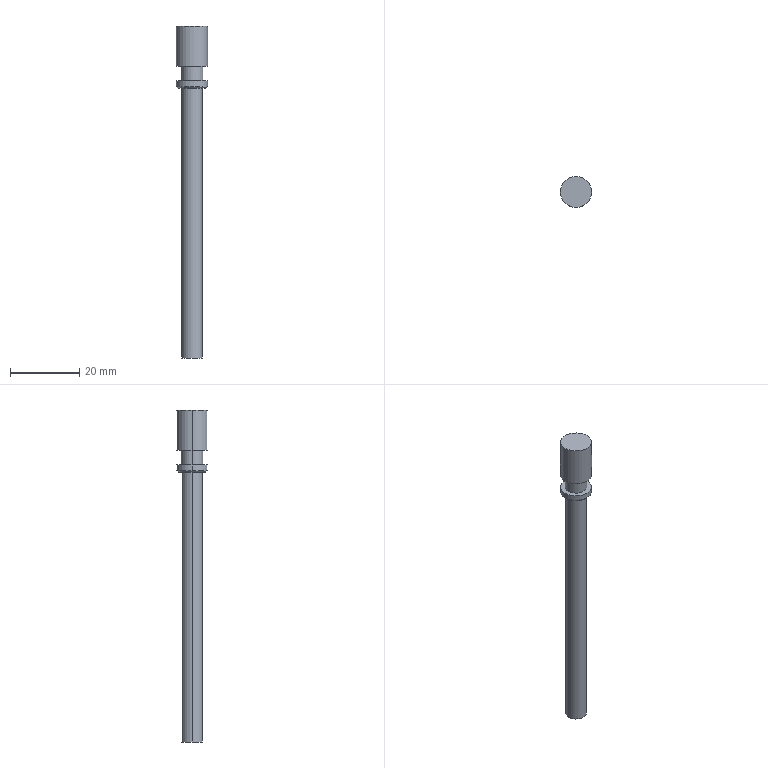Part | SolidWorks | features ICE 2, Chamfer 1, Extrusion 1 | 1 solid | 15 faces | box 9 x 9 x 96 mm | volume 3208 mm3 | cylinder 8 | plane 5 | cone 2 | commonest cylinder face diameters 9 x4 6 x2 6.3 x2
STEP:
#1=CARTESIAN_POINT('',(-4.,0.,78.));
#2=VERTEX_POINT('',#1);
#3=CARTESIAN_POINT('',(4.,0.,78.));
#4=VERTEX_POINT('',#3);
#5=CARTESIAN_POINT('',(0.,0.,78.));
#6=DIRECTION('',(0.,0.,-1.));
#7=DIRECTION('',(1.,0.,0.));
#8=AXIS2_PLACEMENT_3D('',#5,#6,#7);
#9=CIRCLE('',#8,4.);
#10=EDGE_CURVE('',#2,#4,#9,.T.);
#11=ORIENTED_EDGE('',*,*,#10,.F.);
#12=CARTESIAN_POINT('',(-4.5,0.,78.5));
#13=VERTEX_POINT('',#12);
#14=CARTESIAN_POINT('',(-4.5,0.,78.5));
#15=DIRECTION('',(-0.7071,0.,0.7071));
#16=VECTOR('',#15,1000.);
#17=LINE('',#14,#16);
#18=EDGE_CURVE('',#2,#13,#17,.T.);
#19=ORIENTED_EDGE('',*,*,#18,.T.);
#20=CARTESIAN_POINT('',(4.5,0.,78.5));
#21=VERTEX_POINT('',#20);
#22=CARTESIAN_POINT('',(0.,0.,78.5));
#23=DIRECTION('',(0.,0.,1.));
#24=DIRECTION('',(1.,0.,0.));
#25=AXIS2_PLACEMENT_3D('',#22,#23,#24);
#26=CIRCLE('',#25,4.5);
#27=EDGE_CURVE('',#21,#13,#26,.T.);
#28=ORIENTED_EDGE('',*,*,#27,.F.);
#29=CARTESIAN_POINT('',(4.5,0.,78.5));
#30=DIRECTION('',(0.7071,0.,0.7071));
#31=VECTOR('',#30,1000.);
#32=LINE('',#29,#31);
#33=EDGE_CURVE('',#4,#21,#32,.T.);
#34=ORIENTED_EDGE('',*,*,#33,.F.);
#35=EDGE_LOOP('',(#11,#19,#28,#34));
#36=FACE_OUTER_BOUND('',#35,.T.);
#37=CARTESIAN_POINT('',(0.,0.,78.5));
#38=DIRECTION('',(0.,0.,1.));
#39=DIRECTION('',(1.,0.,0.));
#40=AXIS2_PLACEMENT_3D('',#37,#38,#39);
#41=CONICAL_SURFACE('',#40,4.5,0.7854);
#42=ADVANCED_FACE('',(#36),#41,.T.);
#43=CARTESIAN_POINT('',(-4.5,0.,84.4));
#44=VERTEX_POINT('',#43);
#45=CARTESIAN_POINT('',(4.5,0.,84.4));
#46=VERTEX_POINT('',#45);
#47=CARTESIAN_POINT('',(0.,0.,84.4));
#48=DIRECTION('',(0.,0.,-1.));
#49=DIRECTION('',(1.,0.,0.));
#50=AXIS2_PLACEMENT_3D('',#47,#48,#49);
#51=CIRCLE('',#50,4.5);
#52=EDGE_CURVE('',#44,#46,#51,.T.);
#53=ORIENTED_EDGE('',*,*,#52,.F.);
#54=CARTESIAN_POINT('',(-4.5,0.,96.));
#55=VERTEX_POINT('',#54);
#56=CARTESIAN_POINT('',(-4.5,0.,78.));
#57=DIRECTION('',(0.,0.,1.));
#58=VECTOR('',#57,1000.);
#59=LINE('',#56,#58);
#60=EDGE_CURVE('',#44,#55,#59,.T.);
#61=ORIENTED_EDGE('',*,*,#60,.T.);
#62=CARTESIAN_POINT('',(4.5,0.,96.));
#63=VERTEX_POINT('',#62);
#64=CARTESIAN_POINT('',(0.,0.,96.));
#65=DIRECTION('',(0.,0.,1.));
#66=DIRECTION('',(1.,0.,0.));
#67=AXIS2_PLACEMENT_3D('',#64,#65,#66);
#68=CIRCLE('',#67,4.5);
#69=EDGE_CURVE('',#63,#55,#68,.T.);
#70=ORIENTED_EDGE('',*,*,#69,.F.);
#71=CARTESIAN_POINT('',(4.5,0.,78.));
#72=DIRECTION('',(0.,0.,1.));
#73=VECTOR('',#72,1000.);
#74=LINE('',#71,#73);
#75=EDGE_CURVE('',#46,#63,#74,.T.);
#76=ORIENTED_EDGE('',*,*,#75,.F.);
#77=EDGE_LOOP('',(#53,#61,#70,#76));
#78=FACE_OUTER_BOUND('',#77,.T.);
#79=CARTESIAN_POINT('',(0.,0.,78.));
#80=DIRECTION('',(0.,0.,1.));
#81=DIRECTION('',(1.,0.,0.));
#82=AXIS2_PLACEMENT_3D('',#79,#80,#81);
#83=CYLINDRICAL_SURFACE('',#82,4.5);
#84=ADVANCED_FACE('',(#78),#83,.T.);
#85=CARTESIAN_POINT('',(3.15,0.,80.1));
#86=VERTEX_POINT('',#85);
#87=CARTESIAN_POINT('',(-3.15,0.,80.1));
#88=VERTEX_POINT('',#87);
#89=CARTESIAN_POINT('',(0.,0.,80.1));
#90=DIRECTION('',(0.,0.,1.));
#91=DIRECTION('',(1.,0.,0.));
#92=AXIS2_PLACEMENT_3D('',#89,#90,#91);
#93=CIRCLE('',#92,3.15);
#94=EDGE_CURVE('',#86,#88,#93,.T.);
#95=ORIENTED_EDGE('',*,*,#94,.T.);
#96=CARTESIAN_POINT('',(-3.15,0.,84.4));
#97=VERTEX_POINT('',#96);
#98=CARTESIAN_POINT('',(-3.15,0.,80.1));
#99=DIRECTION('',(0.,0.,1.));
#100=VECTOR('',#99,1000.);
#101=LINE('',#98,#100);
#102=EDGE_CURVE('',#88,#97,#101,.T.);
#103=ORIENTED_EDGE('',*,*,#102,.T.);
#104=CARTESIAN_POINT('',(3.15,0.,84.4));
#105=VERTEX_POINT('',#104);
#106=CARTESIAN_POINT('',(0.,0.,84.4));
#107=DIRECTION('',(0.,0.,1.));
#108=DIRECTION('',(1.,0.,0.));
#109=AXIS2_PLACEMENT_3D('',#106,#107,#108);
#110=CIRCLE('',#109,3.15);
#111=EDGE_CURVE('',#105,#97,#110,.T.);
#112=ORIENTED_EDGE('',*,*,#111,.F.);
#113=CARTESIAN_POINT('',(3.15,0.,80.1));
#114=DIRECTION('',(0.,0.,1.));
#115=VECTOR('',#114,1000.);
#116=LINE('',#113,#115);
#117=EDGE_CURVE('',#86,#105,#116,.T.);
#118=ORIENTED_EDGE('',*,*,#117,.F.);
#119=EDGE_LOOP('',(#95,#103,#112,#118));
#120=FACE_OUTER_BOUND('',#119,.T.);
#121=CARTESIAN_POINT('',(0.,0.,80.1));
#122=DIRECTION('',(0.,0.,1.));
#123=DIRECTION('',(1.,0.,0.));
#124=AXIS2_PLACEMENT_3D('',#121,#122,#123);
#125=CYLINDRICAL_SURFACE('',#124,3.15);
#126=ADVANCED_FACE('',(#120),#125,.T.);
#127=CARTESIAN_POINT('',(3.,0.,78.));
#128=VERTEX_POINT('',#127);
#129=CARTESIAN_POINT('',(-3.,0.,78.));
#130=VERTEX_POINT('',#129);
#131=CARTESIAN_POINT('',(0.,0.,78.));
#132=DIRECTION('',(0.,0.,1.));
#133=DIRECTION('',(1.,0.,0.));
#134=AXIS2_PLACEMENT_3D('',#131,#132,#133);
#135=CIRCLE('',#134,3.);
#136=EDGE_CURVE('',#128,#130,#135,.T.);
#137=ORIENTED_EDGE('',*,*,#136,.F.);
#138=CARTESIAN_POINT('',(3.,0.,0.));
#139=VERTEX_POINT('',#138);
#140=CARTESIAN_POINT('',(3.,0.,96.));
#141=DIRECTION('',(0.,0.,-1.));
#142=VECTOR('',#141,1000.);
#143=LINE('',#140,#142);
#144=EDGE_CURVE('',#128,#139,#143,.T.);
#145=ORIENTED_EDGE('',*,*,#144,.T.);
#146=CARTESIAN_POINT('',(-3.,0.,0.));
#147=VERTEX_POINT('',#146);
#148=CARTESIAN_POINT('',(0.,0.,0.));
#149=DIRECTION('',(0.,0.,1.));
#150=DIRECTION('',(1.,0.,0.));
#151=AXIS2_PLACEMENT_3D('',#148,#149,#150);
#152=CIRCLE('',#151,3.);
#153=EDGE_CURVE('',#139,#147,#152,.T.);
#154=ORIENTED_EDGE('',*,*,#153,.T.);
#155=CARTESIAN_POINT('',(-3.,0.,96.));
#156=DIRECTION('',(0.,0.,-1.));
#157=VECTOR('',#156,1000.);
#158=LINE('',#155,#157);
#159=EDGE_CURVE('',#130,#147,#158,.T.);
#160=ORIENTED_EDGE('',*,*,#159,.F.);
#161=EDGE_LOOP('',(#137,#145,#154,#160));
#162=FACE_OUTER_BOUND('',#161,.T.);
#163=CARTESIAN_POINT('',(0.,0.,96.));
#164=DIRECTION('',(0.,0.,-1.));
#165=DIRECTION('',(-1.,0.,0.));
#166=AXIS2_PLACEMENT_3D('',#163,#164,#165);
#167=CYLINDRICAL_SURFACE('',#166,3.);
#168=ADVANCED_FACE('',(#162),#167,.T.);
#169=ORIENTED_EDGE('',*,*,#27,.T.);
#170=CARTESIAN_POINT('',(-4.5,0.,80.1));
#171=VERTEX_POINT('',#170);
#172=CARTESIAN_POINT('',(-4.5,0.,78.));
#173=DIRECTION('',(0.,0.,1.));
#174=VECTOR('',#173,1000.);
#175=LINE('',#172,#174);
#176=EDGE_CURVE('',#13,#171,#175,.T.);
#177=ORIENTED_EDGE('',*,*,#176,.T.);
#178=CARTESIAN_POINT('',(4.5,0.,80.1));
#179=VERTEX_POINT('',#178);
#180=CARTESIAN_POINT('',(0.,0.,80.1));
#181=DIRECTION('',(0.,0.,-1.));
#182=DIRECTION('',(1.,0.,0.));
#183=AXIS2_PLACEMENT_3D('',#180,#181,#182);
#184=CIRCLE('',#183,4.5);
#185=EDGE_CURVE('',#171,#179,#184,.T.);
#186=ORIENTED_EDGE('',*,*,#185,.T.);
#187=CARTESIAN_POINT('',(4.5,0.,78.));
#188=DIRECTION('',(0.,0.,1.));
#189=VECTOR('',#188,1000.);
#190=LINE('',#187,#189);
#191=EDGE_CURVE('',#21,#179,#190,.T.);
#192=ORIENTED_EDGE('',*,*,#191,.F.);
#193=EDGE_LOOP('',(#169,#177,#186,#192));
#194=FACE_OUTER_BOUND('',#193,.T.);
#195=CARTESIAN_POINT('',(0.,0.,78.));
#196=DIRECTION('',(0.,0.,1.));
#197=DIRECTION('',(1.,0.,0.));
#198=AXIS2_PLACEMENT_3D('',#195,#196,#197);
#199=CYLINDRICAL_SURFACE('',#198,4.5);
#200=ADVANCED_FACE('',(#194),#199,.T.);
#201=ORIENTED_EDGE('',*,*,#176,.F.);
#202=CARTESIAN_POINT('',(0.,0.,78.5));
#203=DIRECTION('',(0.,0.,1.));
#204=DIRECTION('',(1.,0.,0.));
#205=AXIS2_PLACEMENT_3D('',#202,#203,#204);
#206=CIRCLE('',#205,4.5);
#207=EDGE_CURVE('',#13,#21,#206,.T.);
#208=ORIENTED_EDGE('',*,*,#207,.T.);
#209=ORIENTED_EDGE('',*,*,#191,.T.);
#210=CARTESIAN_POINT('',(0.,0.,80.1));
#211=DIRECTION('',(0.,0.,-1.));
#212=DIRECTION('',(1.,0.,0.));
#213=AXIS2_PLACEMENT_3D('',#210,#211,#212);
#214=CIRCLE('',#213,4.5);
#215=EDGE_CURVE('',#179,#171,#214,.T.);
#216=ORIENTED_EDGE('',*,*,#215,.T.);
#217=EDGE_LOOP('',(#201,#208,#209,#216));
#218=FACE_OUTER_BOUND('',#217,.T.);
#219=CARTESIAN_POINT('',(0.,0.,78.));
#220=DIRECTION('',(0.,0.,1.));
#221=DIRECTION('',(1.,0.,0.));
#222=AXIS2_PLACEMENT_3D('',#219,#220,#221);
#223=CYLINDRICAL_SURFACE('',#222,4.5);
#224=ADVANCED_FACE('',(#218),#223,.T.);
#225=ORIENTED_EDGE('',*,*,#144,.F.);
#226=CARTESIAN_POINT('',(0.,0.,78.));
#227=DIRECTION('',(0.,0.,1.));
#228=DIRECTION('',(1.,0.,0.));
#229=AXIS2_PLACEMENT_3D('',#226,#227,#228);
#230=CIRCLE('',#229,3.);
#231=EDGE_CURVE('',#130,#128,#230,.T.);
#232=ORIENTED_EDGE('',*,*,#231,.F.);
#233=ORIENTED_EDGE('',*,*,#159,.T.);
#234=CARTESIAN_POINT('',(0.,0.,0.));
#235=DIRECTION('',(0.,0.,1.));
#236=DIRECTION('',(1.,0.,0.));
#237=AXIS2_PLACEMENT_3D('',#234,#235,#236);
#238=CIRCLE('',#237,3.);
#239=EDGE_CURVE('',#147,#139,#238,.T.);
#240=ORIENTED_EDGE('',*,*,#239,.T.);
#241=EDGE_LOOP('',(#225,#232,#233,#240));
#242=FACE_OUTER_BOUND('',#241,.T.);
#243=CARTESIAN_POINT('',(0.,0.,96.));
#244=DIRECTION('',(0.,0.,-1.));
#245=DIRECTION('',(-1.,0.,0.));
#246=AXIS2_PLACEMENT_3D('',#243,#244,#245);
#247=CYLINDRICAL_SURFACE('',#246,3.);
#248=ADVANCED_FACE('',(#242),#247,.T.);
#249=ORIENTED_EDGE('',*,*,#239,.F.);
#250=ORIENTED_EDGE('',*,*,#153,.F.);
#251=EDGE_LOOP('',(#249,#250));
#252=FACE_OUTER_BOUND('',#251,.T.);
#253=CARTESIAN_POINT('',(0.,0.,0.));
#254=DIRECTION('',(0.,0.,1.));
#255=DIRECTION('',(1.,0.,0.));
#256=AXIS2_PLACEMENT_3D('',#253,#254,#255);
#257=PLANE('',#256);
#258=ADVANCED_FACE('',(#252),#257,.F.);
#259=CARTESIAN_POINT('',(0.,0.,78.));
#260=DIRECTION('',(0.,0.,-1.));
#261=DIRECTION('',(1.,0.,0.));
#262=AXIS2_PLACEMENT_3D('',#259,#260,#261);
#263=CIRCLE('',#262,4.);
#264=EDGE_CURVE('',#4,#2,#263,.T.);
#265=ORIENTED_EDGE('',*,*,#264,.T.);
#266=ORIENTED_EDGE('',*,*,#10,.T.);
#267=EDGE_LOOP('',(#265,#266));
#268=FACE_OUTER_BOUND('',#267,.T.);
#269=ORIENTED_EDGE('',*,*,#231,.T.);
#270=ORIENTED_EDGE('',*,*,#136,.T.);
#271=EDGE_LOOP('',(#269,#270));
#272=FACE_BOUND('',#271,.T.);
#273=CARTESIAN_POINT('',(0.,0.,78.));
#274=DIRECTION('',(0.,0.,1.));
#275=DIRECTION('',(1.,0.,0.));
#276=AXIS2_PLACEMENT_3D('',#273,#274,#275);
#277=PLANE('',#276);
#278=ADVANCED_FACE('',(#268,#272),#277,.F.);
#279=ORIENTED_EDGE('',*,*,#215,.F.);
#280=ORIENTED_EDGE('',*,*,#185,.F.);
#281=EDGE_LOOP('',(#279,#280));
#282=FACE_OUTER_BOUND('',#281,.T.);
#283=ORIENTED_EDGE('',*,*,#94,.F.);
#284=CARTESIAN_POINT('',(0.,0.,80.1));
#285=DIRECTION('',(0.,0.,1.));
#286=DIRECTION('',(1.,0.,0.));
#287=AXIS2_PLACEMENT_3D('',#284,#285,#286);
#288=CIRCLE('',#287,3.15);
#289=EDGE_CURVE('',#88,#86,#288,.T.);
#290=ORIENTED_EDGE('',*,*,#289,.F.);
#291=EDGE_LOOP('',(#283,#290));
#292=FACE_BOUND('',#291,.T.);
#293=CARTESIAN_POINT('',(0.,0.,80.1));
#294=DIRECTION('',(0.,0.,1.));
#295=DIRECTION('',(1.,0.,0.));
#296=AXIS2_PLACEMENT_3D('',#293,#294,#295);
#297=PLANE('',#296);
#298=ADVANCED_FACE('',(#282,#292),#297,.T.);
#299=CARTESIAN_POINT('',(0.,0.,84.4));
#300=DIRECTION('',(0.,0.,-1.));
#301=DIRECTION('',(1.,0.,0.));
#302=AXIS2_PLACEMENT_3D('',#299,#300,#301);
#303=CIRCLE('',#302,4.5);
#304=EDGE_CURVE('',#46,#44,#303,.T.);
#305=ORIENTED_EDGE('',*,*,#304,.T.);
#306=ORIENTED_EDGE('',*,*,#52,.T.);
#307=EDGE_LOOP('',(#305,#306));
#308=FACE_OUTER_BOUND('',#307,.T.);
#309=ORIENTED_EDGE('',*,*,#111,.T.);
#310=CARTESIAN_POINT('',(0.,0.,84.4));
#311=DIRECTION('',(0.,0.,1.));
#312=DIRECTION('',(1.,0.,0.));
#313=AXIS2_PLACEMENT_3D('',#310,#311,#312);
#314=CIRCLE('',#313,3.15);
#315=EDGE_CURVE('',#97,#105,#314,.T.);
#316=ORIENTED_EDGE('',*,*,#315,.T.);
#317=EDGE_LOOP('',(#309,#316));
#318=FACE_BOUND('',#317,.T.);
#319=CARTESIAN_POINT('',(0.,0.,84.4));
#320=DIRECTION('',(0.,0.,1.));
#321=DIRECTION('',(1.,0.,0.));
#322=AXIS2_PLACEMENT_3D('',#319,#320,#321);
#323=PLANE('',#322);
#324=ADVANCED_FACE('',(#308,#318),#323,.F.);
#325=ORIENTED_EDGE('',*,*,#102,.F.);
#326=ORIENTED_EDGE('',*,*,#289,.T.);
#327=ORIENTED_EDGE('',*,*,#117,.T.);
#328=ORIENTED_EDGE('',*,*,#315,.F.);
#329=EDGE_LOOP('',(#325,#326,#327,#328));
#330=FACE_OUTER_BOUND('',#329,.T.);
#331=CARTESIAN_POINT('',(0.,0.,80.1));
#332=DIRECTION('',(0.,0.,1.));
#333=DIRECTION('',(1.,0.,0.));
#334=AXIS2_PLACEMENT_3D('',#331,#332,#333);
#335=CYLINDRICAL_SURFACE('',#334,3.15);
#336=ADVANCED_FACE('',(#330),#335,.T.);
#337=ORIENTED_EDGE('',*,*,#69,.T.);
#338=CARTESIAN_POINT('',(0.,0.,96.));
#339=DIRECTION('',(0.,0.,1.));
#340=DIRECTION('',(1.,0.,0.));
#341=AXIS2_PLACEMENT_3D('',#338,#339,#340);
#342=CIRCLE('',#341,4.5);
#343=EDGE_CURVE('',#55,#63,#342,.T.);
#344=ORIENTED_EDGE('',*,*,#343,.T.);
#345=EDGE_LOOP('',(#337,#344));
#346=FACE_OUTER_BOUND('',#345,.T.);
#347=CARTESIAN_POINT('',(0.,0.,96.));
#348=DIRECTION('',(0.,0.,1.));
#349=DIRECTION('',(1.,0.,0.));
#350=AXIS2_PLACEMENT_3D('',#347,#348,#349);
#351=PLANE('',#350);
#352=ADVANCED_FACE('',(#346),#351,.T.);
#353=ORIENTED_EDGE('',*,*,#60,.F.);
#354=ORIENTED_EDGE('',*,*,#304,.F.);
#355=ORIENTED_EDGE('',*,*,#75,.T.);
#356=ORIENTED_EDGE('',*,*,#343,.F.);
#357=EDGE_LOOP('',(#353,#354,#355,#356));
#358=FACE_OUTER_BOUND('',#357,.T.);
#359=CARTESIAN_POINT('',(0.,0.,78.));
#360=DIRECTION('',(0.,0.,1.));
#361=DIRECTION('',(1.,0.,0.));
#362=AXIS2_PLACEMENT_3D('',#359,#360,#361);
#363=CYLINDRICAL_SURFACE('',#362,4.5);
#364=ADVANCED_FACE('',(#358),#363,.T.);
#365=ORIENTED_EDGE('',*,*,#18,.F.);
#366=ORIENTED_EDGE('',*,*,#264,.F.);
#367=ORIENTED_EDGE('',*,*,#33,.T.);
#368=ORIENTED_EDGE('',*,*,#207,.F.);
#369=EDGE_LOOP('',(#365,#366,#367,#368));
#370=FACE_OUTER_BOUND('',#369,.T.);
#371=CARTESIAN_POINT('',(0.,0.,78.5));
#372=DIRECTION('',(0.,0.,1.));
#373=DIRECTION('',(1.,0.,0.));
#374=AXIS2_PLACEMENT_3D('',#371,#372,#373);
#375=CONICAL_SURFACE('',#374,4.5,0.7854);
#376=ADVANCED_FACE('',(#370),#375,.T.);
#377=CLOSED_SHELL('',(#42,#84,#126,#168,#200,#224,#248,#258,#278,#298,#324,#336,#352,#364,#376));
#378=MANIFOLD_SOLID_BREP('',#377);
#379=CARTESIAN_POINT('',(0.,0.,0.));
#380=DIRECTION('',(0.,0.,1.));
#381=DIRECTION('',(1.,0.,0.));
#382=AXIS2_PLACEMENT_3D('',#379,#380,#381);
#383=(LENGTH_UNIT()NAMED_UNIT(*)SI_UNIT(.MILLI.,.METRE.));
#384=UNCERTAINTY_MEASURE_WITH_UNIT(LENGTH_MEASURE(0.00001),#383,'','');
#385=(NAMED_UNIT(*)PLANE_ANGLE_UNIT()SI_UNIT($,.RADIAN.));
#386=(NAMED_UNIT(*)SI_UNIT($,.STERADIAN.)SOLID_ANGLE_UNIT());
#387=(GEOMETRIC_REPRESENTATION_CONTEXT(3)GLOBAL_UNCERTAINTY_ASSIGNED_CONTEXT((#384))GLOBAL_UNIT_ASSIGNED_CONTEXT((#383,#385,#386))REPRESENTATION_CONTEXT('',''));
#388=ADVANCED_BREP_SHAPE_REPRESENTATION('',(#378,#382),#387);